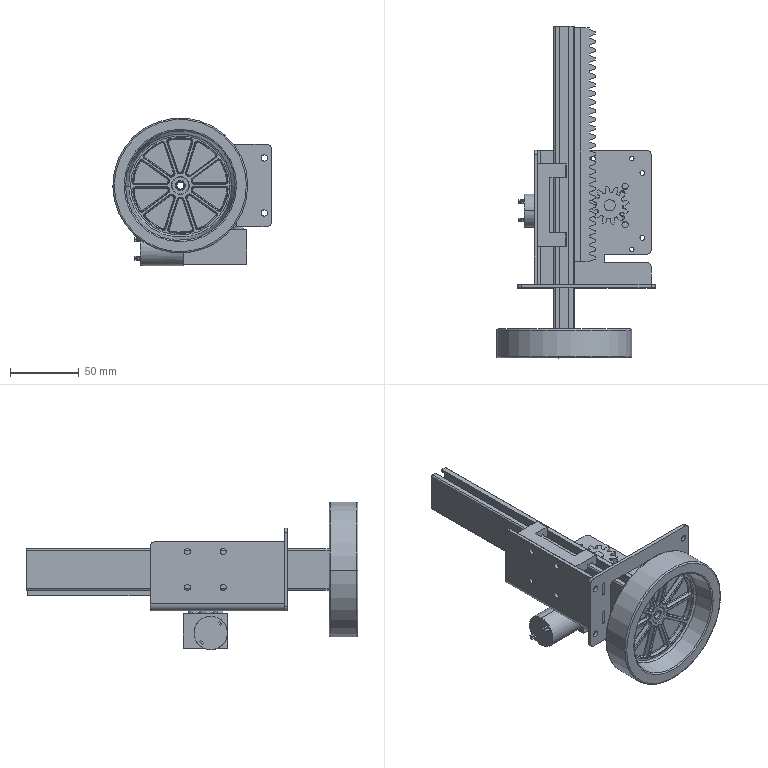Part | SolidWorks | features InContextFeatHolder 17 | 8 solids | 868 faces | box 115 x 241 x 107.2 mm | volume 279061 mm3 | plane 361 | cylinder 323 | torus 148 | spline 24 | cone 12 | commonest cylinder face diameters 1 x56 3 x50 4.5 x40 1.52 x30 3.2 x18 3.3 x16